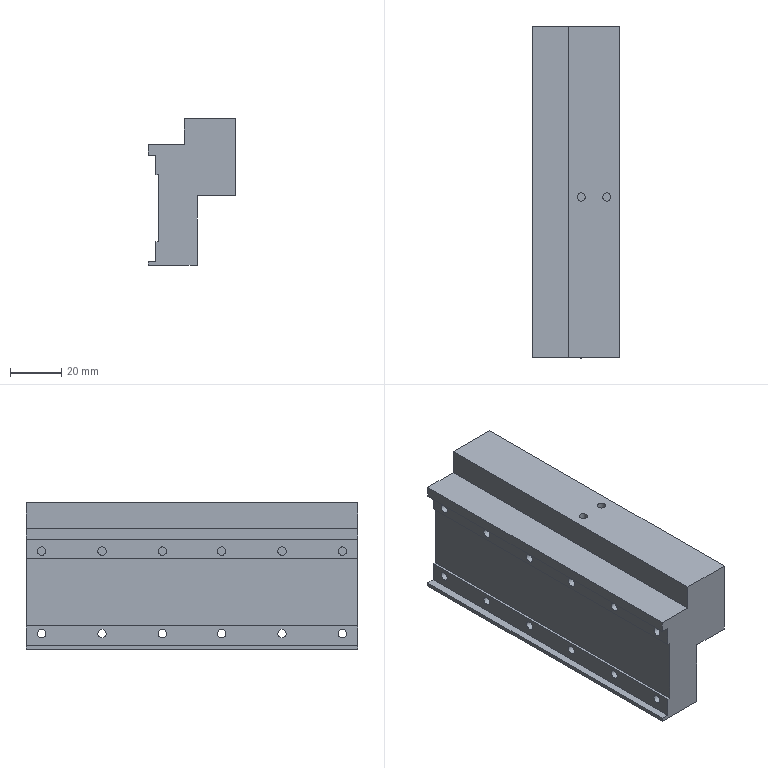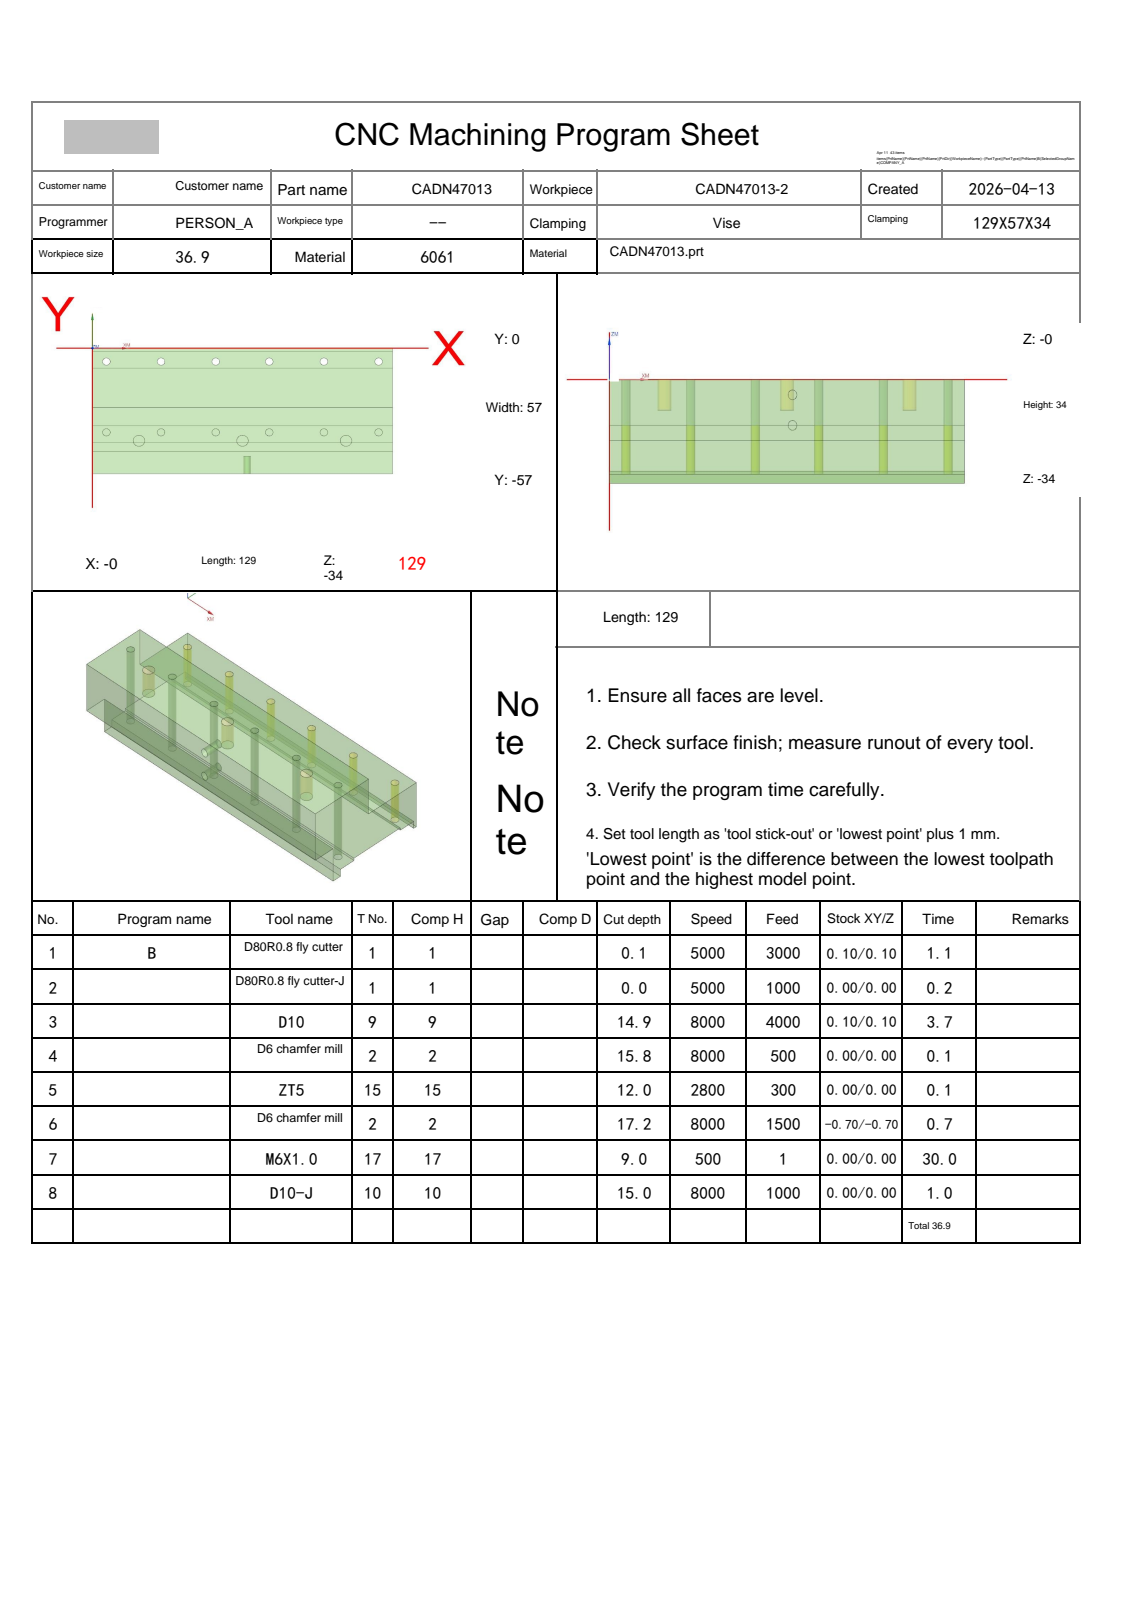NC program | NX | posted by the shop | part box 34 x 129 x 57 mm
Whole program:
%
O0001
(Machine time: 65.54 MIN)
(===Total Tool:6===)
(T1=D80R0.8 fly cutter D=80.  R=0.8  D-  H01 Z=-0.   )
(T9=D10     D=10.  R=0.   D-  H09 Z=-14.9 )
(T2=D6 chamfer mill   D=6.   R=0.   D-  H02 Z=-17.2 )
(T15=ZT5    D=5.   DR_a=118 D-  H15 Z=-12.  )
(T17=M6X1.0 D=5.   DR_a=180 D-  H17 Z=-9.   )
(T10=D10-J  D=10.  R=0.   D10 H10 Z=-15.  )
G80 G90 G17 G49 G40
G91 G28 Z0
M01
N1 T01 M06
(D80R0.8 fly cutter  D=80. R=0.8 H=01 ce=0.10 di=0.10)
G00 G90 G54 X181.097 Y-28.5 M03 S5000
G43 H01 Z20.
M08
Z7.009
G01 Z5.009 F3000.
X169.097
X-40.097
X-52.097
Z7.009
G00 X181.097
Z6.518
G01 Z4.518
X169.097
X-40.097
X-52.097
Z6.518
G00 X181.097
Z6.027
G01 Z4.027
X169.097
X-40.097
X-52.097
Z6.027
G00 X181.097
Z5.536
G01 Z3.536
X169.097
X-40.097
X-52.097
Z5.536
G00 Z20.
X181.097
Z5.045
G01 Z3.045
X169.097
X-40.097
X-52.097
Z5.045
G00 Z20.
X181.097
Z4.555
G01 Z2.555
X169.097
X-40.097
X-52.097
Z4.555
G00 Z20.
X181.097
Z4.064
G01 Z2.064
X169.097
X-40.097
X-52.097
Z4.064
G00 Z20.
X181.097
Z3.573
G01 Z1.573
X169.097
X-40.097
X-52.097
Z3.573
G00 Z20.
X181.097
Z3.082
G01 Z1.082
X169.097
X-40.097
X-52.097
Z3.082
G00 Z20.
X181.097
Z2.591
G01 Z.591
X169.097
X-40.097
X-52.097
Z2.591
G00 Z20.
X181.097
Z2.1
G01 Z.1
X169.097
X-40.097
X-52.097
Z2.1
G00 Z20.
G91 G28 Z0.0
M05
M09
G91 G28 Z0.0
M01
N2 T01 M06
(D80R0.8 fly cutter-J  D=80. R=0.8 H=01 ce=0.00 di=0.00)
G00 G90 G54 X180.999 Y-28.5 M03 S5000
G43 H01 Z20.
M08
Z2.
G01 Z0.0 F1000.
X168.999
X-39.999
X-51.999
Z2.
G00 Z20.
G91 G28 Z0.0
M05
M09
G91 G28 Z0.0
M01
N3 T09 M06
(D10  D=10. R=0. H=09 ce=0.10 di=0.10)
G00 G90 G54 X137. Y.6 M03 S8000
G43 H09 Z15.8
M08
Z.904
G01 Z-.596 F4000.
X133.9
X-3.901
G03 X-4.9 Y-.399 I.001 J-1.
G01 Y-5.901
G03 X-3.901 Y-6.9 I1. J.001
G01 X132.901
G02 X133.9 Y-7.899 I-.001 J-1.
G01 Y-13.401
G02 X132.901 Y-14.4 I-1. J.001
G01 X-4.045
G03 X-5.032 Y-15.245 I.001 J-1.
G01 X-5.888 Y-20.746
X-5.9 Y-20.9
G03 X-4.9 Y-21.9 I1. J0.0
G01 X133.9
X137.1
Z.904
G00 X137. Y.6
Z.308
G01 Z-1.192
X133.9
X-3.901
G03 X-4.9 Y-.399 I.001 J-1.
G01 Y-5.901
G03 X-3.901 Y-6.9 I1. J.001
G01 X132.901
G02 X133.9 Y-7.899 I-.001 J-1.
G01 Y-13.401
G02 X132.901 Y-14.4 I-1. J.001
G01 X-4.045
G03 X-5.032 Y-15.245 I.001 J-1.
G01 X-5.888 Y-20.746
X-5.9 Y-20.9
G03 X-4.9 Y-21.9 I1. J0.0
G01 X133.9
X137.1
Z.308
G00 X137. Y.6
Z-.288
G01 Z-1.788
X133.9
X-3.901
G03 X-4.9 Y-.399 I.001 J-1.
G01 Y-5.901
G03 X-3.901 Y-6.9 I1. J.001
G01 X132.901
G02 X133.9 Y-7.899 I-.001 J-1.
G01 Y-13.401
G02 X132.901 Y-14.4 I-1. J.001
G01 X-4.045
G03 X-5.032 Y-15.245 I.001 J-1.
G01 X-5.888 Y-20.746
X-5.9 Y-20.9
G03 X-4.9 Y-21.9 I1. J0.0
G01 X133.9
X137.1
Z-.288
G00 X137. Y.6
Z-.884
G01 Z-2.384
X133.9
X-3.901
G03 X-4.9 Y-.399 I.001 J-1.
G01 Y-5.901
G03 X-3.901 Y-6.9 I1. J.001
G01 X132.901
G02 X133.9 Y-7.899 I-.001 J-1.
G01 Y-13.401
G02 X132.901 Y-14.4 I-1. J.001
G01 X-4.045
G03 X-5.032 Y-15.245 I.001 J-1.
G01 X-5.888 Y-20.746
X-5.9 Y-20.9
G03 X-4.9 Y-21.9 I1. J0.0
G01 X133.9
X137.1
Z-.884
G00 X137. Y.6
Z-1.48
G01 Z-2.98
X133.9
X-3.901
G03 X-4.9 Y-.399 I.001 J-1.
G01 Y-5.901
G03 X-3.901 Y-6.9 I1. J.001
G01 X132.901
G02 X133.9 Y-7.899 I-.001 J-1.
G01 Y-13.401
G02 X132.901 Y-14.4 I-1. J.001
G01 X-4.045
G03 X-5.032 Y-15.245 I.001 J-1.
G01 X-5.888 Y-20.746
X-5.9 Y-20.9
G03 X-4.9 Y-21.9 I1. J0.0
G01 X133.9
X137.1
Z-1.48
G00 X137. Y.6
Z-2.076
G01 Z-3.576
X133.9
X-3.901
G03 X-4.9 Y-.399 I.001 J-1.
G01 Y-5.901
G03 X-3.901 Y-6.9 I1. J.001
G01 X132.901
G02 X133.9 Y-7.899 I-.001 J-1.
G01 Y-13.401
G02 X132.901 Y-14.4 I-1. J.001
G01 X-4.045
G03 X-5.032 Y-15.245 I.001 J-1.
G01 X-5.888 Y-20.746
X-5.9 Y-20.9
G03 X-4.9 Y-21.9 I1. J0.0
G01 X133.9
X137.1
Z-2.076
G00 X137. Y.6
Z-2.672
G01 Z-4.172
X133.9
X-3.901
G03 X-4.9 Y-.399 I.001 J-1.
G01 Y-5.901
G03 X-3.901 Y-6.9 I1. J.001
G01 X132.901
G02 X133.9 Y-7.899 I-.001 J-1.
G01 Y-13.401
G02 X132.901 Y-14.4 I-1. J.001
G01 X-4.045
G03 X-5.032 Y-15.245 I.001 J-1.
G01 X-5.888 Y-20.746
X-5.9 Y-20.9
G03 X-4.9 Y-21.9 I1. J0.0
G01 X133.9
X137.1
Z-2.672
G00 X137. Y.6
Z-3.268
G01 Z-4.768
X133.9
X-3.901
G03 X-4.9 Y-.399 I.001 J-1.
G01 Y-5.901
G03 X-3.901 Y-6.9 I1. J.001
G01 X132.901
G02 X133.9 Y-7.899 I-.001 J-1.
G01 Y-13.401
G02 X132.901 Y-14.4 I-1. J.001
G01 X-4.045
G03 X-5.032 Y-15.245 I.001 J-1.
G01 X-5.888 Y-20.746
X-5.9 Y-20.9
G03 X-4.9 Y-21.9 I1. J0.0
G01 X133.9
X137.1
Z-3.268
G00 X137. Y.6
Z-3.864
G01 Z-5.364
X133.9
X-3.901
G03 X-4.9 Y-.399 I.001 J-1.
G01 Y-5.901
G03 X-3.901 Y-6.9 I1. J.001
G01 X132.901
G02 X133.9 Y-7.899 I-.001 J-1.
G01 Y-13.401
G02 X132.901 Y-14.4 I-1. J.001
G01 X-4.045
G03 X-5.032 Y-15.245 I.001 J-1.
G01 X-5.888 Y-20.746
X-5.9 Y-20.9
G03 X-4.9 Y-21.9 I1. J0.0
G01 X133.9
X137.1
Z-3.864
G00 X137. Y.6
Z-4.46
G01 Z-5.96
X133.9
X-3.901
G03 X-4.9 Y-.399 I.001 J-1.
G01 Y-5.901
G03 X-3.901 Y-6.9 I1. J.001
G01 X132.901
G02 X133.9 Y-7.899 I-.001 J-1.
G01 Y-13.401
G02 X132.901 Y-14.4 I-1. J.001
G01 X-4.045
G03 X-5.032 Y-15.245 I.001 J-1.
G01 X-5.888 Y-20.746
X-5.9 Y-20.9
G03 X-4.9 Y-21.9 I1. J0.0
G01 X133.9
X137.1
Z-4.46
G00 X137. Y.6
Z-5.056
G01 Z-6.556
X133.9
X-3.901
G03 X-4.9 Y-.399 I.001 J-1.
G01 Y-5.901
G03 X-3.901 Y-6.9 I1. J.001
G01 X132.901
G02 X133.9 Y-7.899 I-.001 J-1.
G01 Y-13.401
G02 X132.901 Y-14.4 I-1. J.001
G01 X-4.045
G03 X-5.032 Y-15.245 I.001 J-1.
G01 X-5.888 Y-20.746
X-5.9 Y-20.9
G03 X-4.9 Y-21.9 I1. J0.0
G01 X133.9
X137.1
Z-5.056
G00 X137. Y.6
Z-5.652
G01 Z-7.152
X133.9
X-3.901
G03 X-4.9 Y-.399 I.001 J-1.
G01 Y-5.901
G03 X-3.901 Y-6.9 I1. J.001
G01 X132.901
G02 X133.9 Y-7.899 I-.001 J-1.
G01 Y-13.401
G02 X132.901 Y-14.4 I-1. J.001
G01 X-4.045
G03 X-5.032 Y-15.245 I.001 J-1.
G01 X-5.888 Y-20.746
X-5.9 Y-20.9
G03 X-4.9 Y-21.9 I1. J0.0
G01 X133.9
X137.1
Z-5.652
G00 X137. Y.6
Z-6.248
G01 Z-7.748
X133.9
X-3.901
G03 X-4.9 Y-.399 I.001 J-1.
G01 Y-5.901
G03 X-3.901 Y-6.9 I1. J.001
G01 X132.901
G02 X133.9 Y-7.899 I-.001 J-1.
G01 Y-13.401
G02 X132.901 Y-14.4 I-1. J.001
G01 X-4.045
G03 X-5.032 Y-15.245 I.001 J-1.
G01 X-5.888 Y-20.746
X-5.9 Y-20.9
G03 X-4.9 Y-21.9 I1. J0.0
G01 X133.9
X137.1
Z-6.248
G00 X137. Y.6
Z-6.844
G01 Z-8.344
X133.9
X-3.901
G03 X-4.9 Y-.399 I.001 J-1.
G01 Y-5.901
G03 X-3.901 Y-6.9 I1. J.001
G01 X132.901
G02 X133.9 Y-7.899 I-.001 J-1.
G01 Y-13.401
G02 X132.901 Y-14.4 I-1. J.001
G01 X-4.045
G03 X-5.032 Y-15.245 I.001 J-1.
G01 X-5.888 Y-20.746
X-5.9 Y-20.9
G03 X-4.9 Y-21.9 I1. J0.0
G01 X133.9
X137.1
Z-6.844
G00 X137. Y.6
Z-7.44
G01 Z-8.94
X133.9
X-3.901
G03 X-4.9 Y-.399 I.001 J-1.
G01 Y-5.901
G03 X-3.901 Y-6.9 I1. J.001
G01 X132.901
G02 X133.9 Y-7.899 I-.001 J-1.
G01 Y-13.401
G02 X132.901 Y-14.4 I-1. J.001
G01 X-4.045
G03 X-5.032 Y-15.245 I.001 J-1.
G01 X-5.888 Y-20.746
X-5.9 Y-20.9
G03 X-4.9 Y-21.9 I1. J0.0
G01 X133.9
X137.1
Z-7.44
G00 X137. Y.6
Z-8.036
G01 Z-9.536
X133.9
X-3.901
G03 X-4.9 Y-.399 I.001 J-1.
G01 Y-5.901
G03 X-3.901 Y-6.9 I1. J.001
G01 X132.901
G02 X133.9 Y-7.899 I-.001 J-1.
G01 Y-13.401
G02 X132.901 Y-14.4 I-1. J.001
G01 X-4.045
G03 X-5.032 Y-15.245 I.001 J-1.
G01 X-5.888 Y-20.746
X-5.9 Y-20.9
G03 X-4.9 Y-21.9 I1. J0.0
G01 X133.9
X137.1
Z-8.036
G00 X137. Y.6
Z-8.632
G01 Z-10.132
X133.9
X-3.901
G03 X-4.9 Y-.399 I.001 J-1.
G01 Y-5.901
G03 X-3.901 Y-6.9 I1. J.001
G01 X132.901
G02 X133.9 Y-7.899 I-.001 J-1.
G01 Y-13.401
G02 X132.901 Y-14.4 I-1. J.001
G01 X-4.045
G03 X-5.032 Y-15.245 I.001 J-1.
G01 X-5.888 Y-20.746
X-5.9 Y-20.9
G03 X-4.9 Y-21.9 I1. J0.0
G01 X133.9
X137.1
Z-8.632
G00 X137. Y.6
Z-9.228
G01 Z-10.728
X133.9
X-3.901
G03 X-4.9 Y-.399 I.001 J-1.
G01 Y-5.901
G03 X-3.901 Y-6.9 I1. J.001
G01 X132.901
G02 X133.9 Y-7.899 I-.001 J-1.
G01 Y-13.401
G02 X132.901 Y-14.4 I-1. J.001
G01 X-4.045
G03 X-5.032 Y-15.245 I.001 J-1.
G01 X-5.888 Y-20.746
X-5.9 Y-20.9
G03 X-4.9 Y-21.9 I1. J0.0
G01 X133.9
X137.1
Z-9.228
G00 X137. Y.6
Z-9.824
G01 Z-11.324
X133.9
X-3.901
G03 X-4.9 Y-.399 I.001 J-1.
G01 Y-5.901
G03 X-3.901 Y-6.9 I1. J.001
G01 X132.901
G02 X133.9 Y-7.899 I-.001 J-1.
G01 Y-13.401
G02 X132.901 Y-14.4 I-1. J.001
G01 X-4.045
G03 X-5.032 Y-15.245 I.001 J-1.
G01 X-5.888 Y-20.746
X-5.9 Y-20.9
G03 X-4.9 Y-21.9 I1. J0.0
G01 X133.9
X137.1
Z-9.824
G00 X137. Y.6
Z-10.42
G01 Z-11.92
X133.9
X-3.901
G03 X-4.9 Y-.399 I.001 J-1.
G01 Y-5.901
G03 X-3.901 Y-6.9 I1. J.001
G01 X132.901
G02 X133.9 Y-7.899 I-.001 J-1.
G01 Y-13.401
G02 X132.901 Y-14.4 I-1. J.001
G01 X-4.045
G03 X-5.032 Y-15.245 I.001 J-1.
G01 X-5.888 Y-20.746
X-5.9 Y-20.9
G03 X-4.9 Y-21.9 I1. J0.0
G01 X133.9
X137.1
Z-10.42
G00 X137. Y.6
Z-11.016
G01 Z-12.516
X133.9
X-3.901
G03 X-4.9 Y-.399 I.001 J-1.
G01 Y-5.901
G03 X-3.901 Y-6.9 I1. J.001
G01 X132.901
G02 X133.9 Y-7.899 I-.001 J-1.
G01 Y-13.401
G02 X132.901 Y-14.4 I-1. J.001
G01 X-4.045
G03 X-5.032 Y-15.245 I.001 J-1.
G01 X-5.888 Y-20.746
X-5.9 Y-20.9
G03 X-4.9 Y-21.9 I1. J0.0
G01 X133.9
X137.1
Z-11.016
G00 X137. Y.6
Z-11.612
G01 Z-13.112
X133.9
X-3.901
G03 X-4.9 Y-.399 I.001 J-1.
G01 Y-5.901
G03 X-3.901 Y-6.9 I1. J.001
G01 X132.901
G02 X133.9 Y-7.899 I-.001 J-1.
G01 Y-13.401
G02 X132.901 Y-14.4 I-1. J.001
G01 X-4.045
G03 X-5.032 Y-15.245 I.001 J-1.
G01 X-5.888 Y-20.746
X-5.9 Y-20.9
G03 X-4.9 Y-21.9 I1. J0.0
G01 X133.9
X137.1
Z-11.612
G00 X137. Y.6
Z-12.208
G01 Z-13.708
X133.9
X-3.901
G03 X-4.9 Y-.399 I.001 J-1.
G01 Y-5.901
G03 X-3.901 Y-6.9 I1. J.001
G01 X132.901
G02 X133.9 Y-7.899 I-.001 J-1.
G01 Y-13.401
G02 X132.901 Y-14.4 I-1. J.001
G01 X-4.045
G03 X-5.032 Y-15.245 I.001 J-1.
G01 X-5.888 Y-20.746
X-5.9 Y-20.9
G03 X-4.9 Y-21.9 I1. J0.0
G01 X133.9
X137.1
Z-12.208
G00 X137. Y.6
Z-12.804
G01 Z-14.304
X133.9
X-3.901
G03 X-4.9 Y-.399 I.001 J-1.
G01 Y-5.901
G03 X-3.901 Y-6.9 I1. J.001
G01 X132.901
G02 X133.9 Y-7.899 I-.001 J-1.
G01 Y-13.401
G02 X132.901 Y-14.4 I-1. J.001
G01 X-4.045
G03 X-5.032 Y-15.245 I.001 J-1.
G01 X-5.888 Y-20.746
X-5.9 Y-20.9
G03 X-4.9 Y-21.9 I1. J0.0
G01 X133.9
X137.1
Z-12.804
G00 X137. Y.6
Z-13.4
G01 Z-14.9
X133.9
X-3.901
G03 X-4.9 Y-.399 I.001 J-1.
G01 Y-5.901
G03 X-3.901 Y-6.9 I1. J.001
G01 X132.901
G02 X133.9 Y-7.899 I-.001 J-1.
G01 Y-13.401
G02 X132.901 Y-14.4 I-1. J.001
G01 X-4.045
G03 X-5.032 Y-15.245 I.001 J-1.
G01 X-5.888 Y-20.746
X-5.9 Y-20.9
G03 X-4.9 Y-21.9 I1. J0.0
G01 X133.9
X137.1
Z-13.4
G00 Z15.8
G91 G28 Z0.0
M05
M09
G91 G28 Z0.0
M01
N4 T02 M06
(D6 chamfer mill  D=6. R=0. H=02 ce=0.00 di=0.10)
G00 G90 G54 X123. Y-6.073 M03 S8000
G43 H02 Z20.
M08
G98 G81 X123. Y-6.073 Z-15.8 R-14. F500.
X99.5
X76.
X53.
X29.5
X6.
X20. Y-42. Z-.8 R1.
X64.5
X109.
G80
G00 Z20.
G91 G28 Z0.0
M05
M09
G91 G28 Z0.0
M01
N5 T15 M06
(ZT5 D=5. DR_a=118 H=15)
G00 G90 G54 X109. Y-42. M03 S2800
G43 H15 Z20.
M08
G98 G83 X109. Y-42. Z-12. R1. F300. Q2.
X64.5
X20.
G80
G00 Z20.
G91 G28 Z0.0
M05
M09
G91 G28 Z0.0
M01
N6 T02 M06
(D6 chamfer mill  D=6. R=0. H=02 ce=0.00 di=0.10)
G00 G90 G54 X123. Y-6.073 M03 S8000
G43 H02 Z20.
M08
G98 G81 X123. Y-6.073 Z-17.2 R-12. F500.
X99.5
X76.
X53.
X29.5
X6.
G80
G00 Z20.
G00 G90 X109.949 Y-41.684 M03 S8000
Z20.
Z-.7
G01 Z-1.2 F500.
X110.5 Y-41.5
G03 X109. Y-40. I-1.5 J0.0
X107. Y-42. I0.0 J-2.
X109. Y-44. I2. J0.0
X111. Y-42. I0.0 J2.
X109. Y-40. I-2. J0.0
X107.5 Y-41.5 I0.0 J-1.5
G01 X108.051 Y-41.684
Z-.7
G00 Z20.
X65.449
Z-.7
G01 Z-1.2
X66. Y-41.5
G03 X64.5 Y-40. I-1.5 J0.0
X62.5 Y-42. I0.0 J-2.
X64.5 Y-44. I2. J0.0
X66.5 Y-42. I0.0 J2.
X64.5 Y-40. I-2. J0.0
X63. Y-41.5 I0.0 J-1.5
G01 X63.551 Y-41.684
Z-.7
G00 Z20.
X20.949
Z-.7
G01 Z-1.2
X21.5 Y-41.5
G03 X20. Y-40. I-1.5 J0.0
X18. Y-42. I0.0 J-2.
X20. Y-44. I2. J0.0
X22. Y-42. I0.0 J2.
X20. Y-40. I-2. J0.0
X18.5 Y-41.5 I0.0 J-1.5
G01 X19.051 Y-41.684
Z-.7
G00 Z20.
G00 G90 X64.114 Y-25.773 M03 S6500
Z20.
Z.172
G01 Z-1.2 F1500.
G03 X64.4 Y-25.973 I1.286 J1.532
G01 X64.446 Y-26.003
X64.5 Y-26.
X129.
G02 X130. Y-27. I0.0 J-1.
G01 Y-57.
G02 X129. Y-58. I-1. J0.0
G01 X0.0
G02 X-1. Y-57. I0.0 J1.
G01 Y-27.
G02 X0.0 Y-26. I1. J0.0
G01 X64.5
X64.554 Y-26.003
X64.6 Y-25.973
G03 X64.886 Y-25.773 I-1. J1.732
G01 Z.172
G00 Z10.
X109.407 Y-40.685
Z.284
G01 Z-1.2
G03 X109.102 Y-40.516 I-1.118 J-1.658
G01 X109.054 Y-40.491
X109. Y-40.5
G03 X107.5 Y-42. I0.0 J-1.5
X109. Y-43.5 I1.5 J0.0
X110.5 Y-42. I0.0 J1.5
X109. Y-40.5 I-1.5 J0.0
G01 X108.946 Y-40.491
X108.898 Y-40.516
G03 X108.593 Y-40.685 I.813 J-1.827
G01 Z.284
G00 Z10.
X64.907
Z.284
G01 Z-1.2
G03 X64.602 Y-40.516 I-1.118 J-1.658
G01 X64.554 Y-40.491
X64.5 Y-40.5
G03 X63. Y-42. I0.0 J-1.5
X64.5 Y-43.5 I1.5 J0.0
X66. Y-42. I0.0 J1.5
X64.5 Y-40.5 I-1.5 J0.0
G01 X64.446 Y-40.491
X64.398 Y-40.516
G03 X64.093 Y-40.685 I.813 J-1.827
G01 Z.284
G00 Z10.
X20.407
Z.284
G01 Z-1.2
G03 X20.102 Y-40.516 I-1.118 J-1.658
G01 X20.054 Y-40.491
X20. Y-40.5
G03 X18.5 Y-42. I0.0 J-1.5
X20. Y-43.5 I1.5 J0.0
X21.5 Y-42. I0.0 J1.5
X20. Y-40.5 I-1.5 J0.0
G01 X19.946 Y-40.491
X19.898 Y-40.516
G03 X19.593 Y-40.685 I.813 J-1.827
G01 Z.284
G00 Z10.
X-1.068 Y-23.978
Z-1.807
G01 Z-16.2
X-1.008 Y-23.892
X-1. Y-23.862
Y0.0
G02 X0.0 Y1. I1. J0.0
G01 X129.
G02 X130. Y0.0 I0.0 J-1.
G01 Y-23.862
X130.008 Y-23.892
X130.068 Y-23.978
Z-1.807
G00 Z10.
X123.419 Y-5.579
Z-14.595
G01 Z-16.2
G03 X123.103 Y-5.432 I-1. J-1.732
G01 X123.053 Y-5.411
X123. Y-5.423
G03 X122.35 Y-6.073 I0.0 J-.65
X123. Y-6.723 I.65 J0.0
X123.65 Y-6.073 I0.0 J.65
X123. Y-5.423 I-.65 J0.0
G01 X122.947 Y-5.411
X122.897 Y-5.432
G03 X122.581 Y-5.579 I.684 J-1.879
G01 Z-14.595
G00 Z10.
X99.919
Z-14.595
G01 Z-16.2
G03 X99.603 Y-5.432 I-1. J-1.732
G01 X99.553 Y-5.411
X99.5 Y-5.423
G03 X98.85 Y-6.073 I0.0 J-.65
X99.5 Y-6.723 I.65 J0.0
X100.15 Y-6.073 I0.0 J.65
X99.5 Y-5.423 I-.65 J0.0
G01 X99.447 Y-5.411
X99.397 Y-5.432
G03 X99.081 Y-5.579 I.684 J-1.879
G01 Z-14.595
G00 Z10.
X76.419
Z-14.595
G01 Z-16.2
G03 X76.103 Y-5.432 I-1. J-1.732
G01 X76.053 Y-5.411
X76. Y-5.423
G03 X75.35 Y-6.073 I0.0 J-.65
X76. Y-6.723 I.65 J0.0
X76.65 Y-6.073 I0.0 J.65
X76. Y-5.423 I-.65 J0.0
G01 X75.947 Y-5.411
X75.897 Y-5.432
G03 X75.581 Y-5.579 I.684 J-1.879
G01 Z-14.595
G00 Z10.
X53.419
Z-14.595
G01 Z-16.2
G03 X53.103 Y-5.432 I-1. J-1.732
G01 X53.053 Y-5.411
X53. Y-5.423
G03 X52.35 Y-6.073 I0.0 J-.65
X53. Y-6.723 I.65 J0.0
X53.65 Y-6.073 I0.0 J.65
X53. Y-5.423 I-.65 J0.0
G01 X52.947 Y-5.411
X52.897 Y-5.432
G03 X52.581 Y-5.579 I.684 J-1.879
G01 Z-14.595
G00 Z10.
X29.919
Z-14.595
G01 Z-16.2
G03 X29.603 Y-5.432 I-1. J-1.732
G01 X29.553 Y-5.411
X29.5 Y-5.423
G03 X28.85 Y-6.073 I0.0 J-.65
X29.5 Y-6.723 I.65 J0.0
X30.15 Y-6.073 I0.0 J.65
X29.5 Y-5.423 I-.65 J0.0
G01 X29.447 Y-5.411
X29.397 Y-5.432
G03 X29.081 Y-5.579 I.684 J-1.879
G01 Z-14.595
G00 Z10.
X6.419
Z-14.595
G01 Z-16.2
G03 X6.103 Y-5.432 I-1. J-1.732
G01 X6.053 Y-5.411
X6. Y-5.423
G03 X5.35 Y-6.073 I0.0 J-.65
X6. Y-6.723 I.65 J0.0
X6.65 Y-6.073 I0.0 J.65
X6. Y-5.423 I-.65 J0.0
G01 X5.947 Y-5.411
X5.897 Y-5.432
G03 X5.581 Y-5.579 I.684 J-1.879
G01 Z-14.595
G00 Z20.
G91 G28 Z0.0
M05
M09
G91 G28 Z0.0
M01
N7 T17 M06
(M6X1.0 D=5. DR_a=180 H=17)
G00 G90 G54 X109. Y-42. M03 S500
G43 H17 Z20.
M08
G95
G98 G84 X109. Y-42. Z-9. R1. F1. Q3.
X64.5
X20.
G80
G94
G00 Z20.
G91 G28 Z0.0
M05
M09
G91 G28 Z0.0
M01
N8 T10 M06
(D10-J  D=10. R=0. H=10 ce=0.40 di=0.00)
G00 G90 G54 X-7. Y2.999 M03 S8000
G43 H10 Z15.8
M08
Z-13.5
G01 Z-15. F1000.
G03 X-5. Y1. I2. J.001
G01 X133.1
G02 X134. Y.1 I0.0 J-.9
G01 Y-2.52
G02 X133. Y-3.52 I-1. J0.0
G01 X-4.1
G03 X-5. Y-4.42 I0.0 J-.9
G01 Y-7.04
G03 X-4. Y-8.04 I1. J0.0
G01 X133.1
G02 X134. Y-8.94 I0.0 J-.9
G01 Y-11.56
G02 X133. Y-12.56 I-1. J0.0
G01 X-4.1
G03 X-5. Y-13.46 I0.0 J-.9
G01 Y-16.08
G03 X-4. Y-17.08 I1. J0.0
G01 X133.1
G02 X134. Y-17.98 I0.0 J-.9
G01 Y-20.6
G02 X133. Y-21.6 I-1. J0.0
G01 X-5.
G02 X-7. Y-19.6 I0.0 J2.
G01 Z-13.5
G00 Z15.8
G00 G90 X-7. Y-19.801 M03 S8000
Z15.8
Z-14.
G01 Z-15. F1000.
G41 D10
Y-20.001
G03 X-5. Y-22. I2. J.001
G01 X134.
G03 X136. Y-20.001 I0.0 J2.
G01 G40 Y-19.801
Z-14.
G00 Z15.8
M05
M09
G91 G28 Z0.0
G91 G28 Y0.0
M30
%